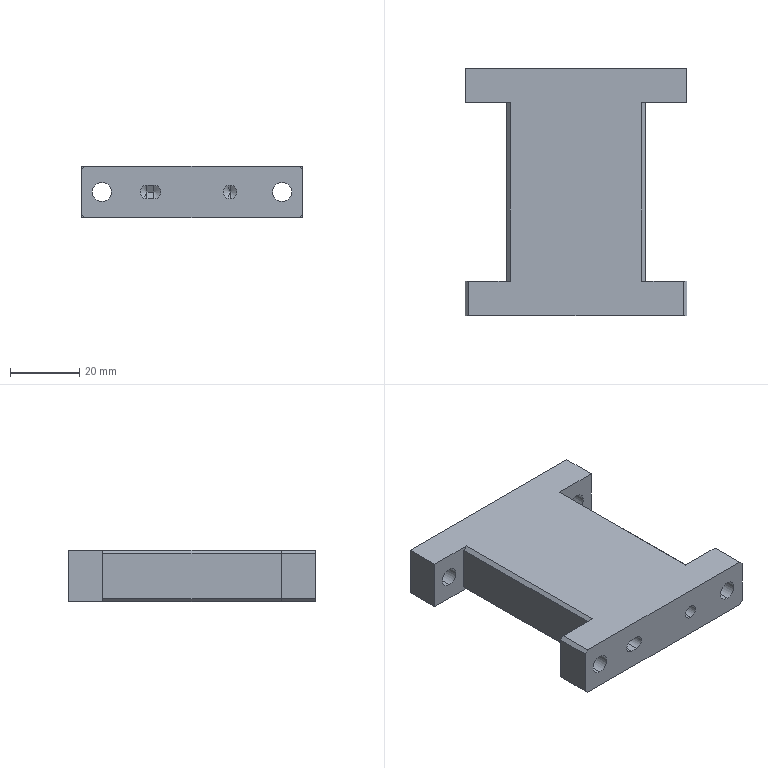Part | STEP file | 11-FG-GD00111 | 1 solid | 42 faces | box 64 x 71.5 x 15 mm | volume 48677 mm3 | plane 26 | cylinder 12 | cone 4 | commonest cylinder face diameters 5.5 x8 4 x4
STEP:
#1=CARTESIAN_POINT('',(26.,35.75,10.25));
#2=VERTEX_POINT('',#1);
#3=CARTESIAN_POINT('',(26.,35.75,4.75));
#4=VERTEX_POINT('',#3);
#5=CARTESIAN_POINT('',(26.,35.75,7.5));
#6=DIRECTION('',(0.,-1.,0.));
#7=DIRECTION('',(0.,0.,-1.));
#8=AXIS2_PLACEMENT_3D('',#5,#6,#7);
#9=CIRCLE('',#8,2.75);
#10=EDGE_CURVE('',#2,#4,#9,.T.);
#11=ORIENTED_EDGE('',*,*,#10,.F.);
#12=CARTESIAN_POINT('',(26.,25.75,10.25));
#13=VERTEX_POINT('',#12);
#14=CARTESIAN_POINT('',(26.,35.75,10.25));
#15=DIRECTION('',(0.,-1.,0.));
#16=VECTOR('',#15,1000.);
#17=LINE('',#14,#16);
#18=EDGE_CURVE('',#2,#13,#17,.T.);
#19=ORIENTED_EDGE('',*,*,#18,.T.);
#20=CARTESIAN_POINT('',(26.,25.75,4.75));
#21=VERTEX_POINT('',#20);
#22=CARTESIAN_POINT('',(26.,25.75,7.5));
#23=DIRECTION('',(0.,-1.,0.));
#24=DIRECTION('',(0.,0.,-1.));
#25=AXIS2_PLACEMENT_3D('',#22,#23,#24);
#26=CIRCLE('',#25,2.75);
#27=EDGE_CURVE('',#13,#21,#26,.T.);
#28=ORIENTED_EDGE('',*,*,#27,.T.);
#29=CARTESIAN_POINT('',(26.,35.75,4.75));
#30=DIRECTION('',(0.,-1.,0.));
#31=VECTOR('',#30,1000.);
#32=LINE('',#29,#31);
#33=EDGE_CURVE('',#4,#21,#32,.T.);
#34=ORIENTED_EDGE('',*,*,#33,.F.);
#35=EDGE_LOOP('',(#11,#19,#28,#34));
#36=FACE_OUTER_BOUND('',#35,.T.);
#37=CARTESIAN_POINT('',(26.,35.75,7.5));
#38=DIRECTION('',(0.,-1.,0.));
#39=DIRECTION('',(0.,0.,-1.));
#40=AXIS2_PLACEMENT_3D('',#37,#38,#39);
#41=CYLINDRICAL_SURFACE('',#40,2.75);
#42=ADVANCED_FACE('',(#36),#41,.F.);
#43=CARTESIAN_POINT('',(-26.,35.75,10.25));
#44=VERTEX_POINT('',#43);
#45=CARTESIAN_POINT('',(-26.,35.75,4.75));
#46=VERTEX_POINT('',#45);
#47=CARTESIAN_POINT('',(-26.,35.75,7.5));
#48=DIRECTION('',(0.,-1.,0.));
#49=DIRECTION('',(0.,0.,-1.));
#50=AXIS2_PLACEMENT_3D('',#47,#48,#49);
#51=CIRCLE('',#50,2.75);
#52=EDGE_CURVE('',#44,#46,#51,.T.);
#53=ORIENTED_EDGE('',*,*,#52,.F.);
#54=CARTESIAN_POINT('',(-26.,25.75,10.25));
#55=VERTEX_POINT('',#54);
#56=CARTESIAN_POINT('',(-26.,35.75,10.25));
#57=DIRECTION('',(0.,-1.,0.));
#58=VECTOR('',#57,1000.);
#59=LINE('',#56,#58);
#60=EDGE_CURVE('',#44,#55,#59,.T.);
#61=ORIENTED_EDGE('',*,*,#60,.T.);
#62=CARTESIAN_POINT('',(-26.,25.75,4.75));
#63=VERTEX_POINT('',#62);
#64=CARTESIAN_POINT('',(-26.,25.75,7.5));
#65=DIRECTION('',(0.,-1.,0.));
#66=DIRECTION('',(0.,0.,-1.));
#67=AXIS2_PLACEMENT_3D('',#64,#65,#66);
#68=CIRCLE('',#67,2.75);
#69=EDGE_CURVE('',#55,#63,#68,.T.);
#70=ORIENTED_EDGE('',*,*,#69,.T.);
#71=CARTESIAN_POINT('',(-26.,35.75,4.75));
#72=DIRECTION('',(0.,-1.,0.));
#73=VECTOR('',#72,1000.);
#74=LINE('',#71,#73);
#75=EDGE_CURVE('',#46,#63,#74,.T.);
#76=ORIENTED_EDGE('',*,*,#75,.F.);
#77=EDGE_LOOP('',(#53,#61,#70,#76));
#78=FACE_OUTER_BOUND('',#77,.T.);
#79=CARTESIAN_POINT('',(-26.,35.75,7.5));
#80=DIRECTION('',(0.,-1.,0.));
#81=DIRECTION('',(0.,0.,-1.));
#82=AXIS2_PLACEMENT_3D('',#79,#80,#81);
#83=CYLINDRICAL_SURFACE('',#82,2.75);
#84=ADVANCED_FACE('',(#78),#83,.F.);
#85=CARTESIAN_POINT('',(11.,-25.65,9.5));
#86=VERTEX_POINT('',#85);
#87=CARTESIAN_POINT('',(11.,-25.65,5.5));
#88=VERTEX_POINT('',#87);
#89=CARTESIAN_POINT('',(11.,-25.65,7.5));
#90=DIRECTION('',(0.,-1.,0.));
#91=DIRECTION('',(0.,0.,-1.));
#92=AXIS2_PLACEMENT_3D('',#89,#90,#91);
#93=CIRCLE('',#92,2.);
#94=EDGE_CURVE('',#86,#88,#93,.T.);
#95=ORIENTED_EDGE('',*,*,#94,.F.);
#96=CARTESIAN_POINT('',(11.,-35.75,9.5));
#97=VERTEX_POINT('',#96);
#98=CARTESIAN_POINT('',(11.,-35.75,9.5));
#99=DIRECTION('',(0.,-1.,0.));
#100=VECTOR('',#99,1000.);
#101=LINE('',#98,#100);
#102=EDGE_CURVE('',#86,#97,#101,.T.);
#103=ORIENTED_EDGE('',*,*,#102,.T.);
#104=CARTESIAN_POINT('',(11.,-35.75,5.5));
#105=VERTEX_POINT('',#104);
#106=CARTESIAN_POINT('',(11.,-35.75,7.5));
#107=DIRECTION('',(0.,-1.,0.));
#108=DIRECTION('',(0.,0.,-1.));
#109=AXIS2_PLACEMENT_3D('',#106,#107,#108);
#110=CIRCLE('',#109,2.);
#111=EDGE_CURVE('',#97,#105,#110,.T.);
#112=ORIENTED_EDGE('',*,*,#111,.T.);
#113=CARTESIAN_POINT('',(11.,-35.75,5.5));
#114=DIRECTION('',(0.,-1.,0.));
#115=VECTOR('',#114,1000.);
#116=LINE('',#113,#115);
#117=EDGE_CURVE('',#88,#105,#116,.T.);
#118=ORIENTED_EDGE('',*,*,#117,.F.);
#119=EDGE_LOOP('',(#95,#103,#112,#118));
#120=FACE_OUTER_BOUND('',#119,.T.);
#121=CARTESIAN_POINT('',(11.,-35.75,7.5));
#122=DIRECTION('',(0.,-1.,0.));
#123=DIRECTION('',(0.,0.,-1.));
#124=AXIS2_PLACEMENT_3D('',#121,#122,#123);
#125=CYLINDRICAL_SURFACE('',#124,2.);
#126=ADVANCED_FACE('',(#120),#125,.F.);
#127=CARTESIAN_POINT('',(11.,-24.448,7.5));
#128=VERTEX_POINT('',#127);
#129=CARTESIAN_POINT('',(11.,-25.65,5.5));
#130=DIRECTION('',(0.,-0.515,-0.8572));
#131=VECTOR('',#130,1000.);
#132=LINE('',#129,#131);
#133=EDGE_CURVE('',#128,#88,#132,.T.);
#134=ORIENTED_EDGE('',*,*,#133,.F.);
#135=CARTESIAN_POINT('',(11.,-25.65,9.5));
#136=DIRECTION('',(0.,-0.515,0.8572));
#137=VECTOR('',#136,1000.);
#138=LINE('',#135,#137);
#139=EDGE_CURVE('',#128,#86,#138,.T.);
#140=ORIENTED_EDGE('',*,*,#139,.T.);
#141=ORIENTED_EDGE('',*,*,#94,.T.);
#142=EDGE_LOOP('',(#134,#140,#141));
#143=FACE_OUTER_BOUND('',#142,.T.);
#144=CARTESIAN_POINT('',(11.,-25.65,7.5));
#145=DIRECTION('',(0.,-1.,0.));
#146=DIRECTION('',(0.,0.,-1.));
#147=AXIS2_PLACEMENT_3D('',#144,#145,#146);
#148=CONICAL_SURFACE('',#147,2.,1.03);
#149=ADVANCED_FACE('',(#143),#148,.F.);
#150=CARTESIAN_POINT('',(26.,-35.75,4.75));
#151=VERTEX_POINT('',#150);
#152=CARTESIAN_POINT('',(26.,-35.75,10.25));
#153=VERTEX_POINT('',#152);
#154=CARTESIAN_POINT('',(26.,-35.75,7.5));
#155=DIRECTION('',(0.,1.,0.));
#156=DIRECTION('',(0.,0.,-1.));
#157=AXIS2_PLACEMENT_3D('',#154,#155,#156);
#158=CIRCLE('',#157,2.75);
#159=EDGE_CURVE('',#151,#153,#158,.T.);
#160=ORIENTED_EDGE('',*,*,#159,.F.);
#161=CARTESIAN_POINT('',(26.,-25.75,4.75));
#162=VERTEX_POINT('',#161);
#163=CARTESIAN_POINT('',(26.,-35.75,4.75));
#164=DIRECTION('',(0.,1.,0.));
#165=VECTOR('',#164,1000.);
#166=LINE('',#163,#165);
#167=EDGE_CURVE('',#151,#162,#166,.T.);
#168=ORIENTED_EDGE('',*,*,#167,.T.);
#169=CARTESIAN_POINT('',(26.,-25.75,10.25));
#170=VERTEX_POINT('',#169);
#171=CARTESIAN_POINT('',(26.,-25.75,7.5));
#172=DIRECTION('',(0.,1.,0.));
#173=DIRECTION('',(0.,0.,-1.));
#174=AXIS2_PLACEMENT_3D('',#171,#172,#173);
#175=CIRCLE('',#174,2.75);
#176=EDGE_CURVE('',#162,#170,#175,.T.);
#177=ORIENTED_EDGE('',*,*,#176,.T.);
#178=CARTESIAN_POINT('',(26.,-35.75,10.25));
#179=DIRECTION('',(0.,1.,0.));
#180=VECTOR('',#179,1000.);
#181=LINE('',#178,#180);
#182=EDGE_CURVE('',#153,#170,#181,.T.);
#183=ORIENTED_EDGE('',*,*,#182,.F.);
#184=EDGE_LOOP('',(#160,#168,#177,#183));
#185=FACE_OUTER_BOUND('',#184,.T.);
#186=CARTESIAN_POINT('',(26.,-35.75,7.5));
#187=DIRECTION('',(0.,1.,0.));
#188=DIRECTION('',(0.,0.,1.));
#189=AXIS2_PLACEMENT_3D('',#186,#187,#188);
#190=CYLINDRICAL_SURFACE('',#189,2.75);
#191=ADVANCED_FACE('',(#185),#190,.F.);
#192=CARTESIAN_POINT('',(-26.,-35.75,4.75));
#193=VERTEX_POINT('',#192);
#194=CARTESIAN_POINT('',(-26.,-35.75,10.25));
#195=VERTEX_POINT('',#194);
#196=CARTESIAN_POINT('',(-26.,-35.75,7.5));
#197=DIRECTION('',(0.,1.,0.));
#198=DIRECTION('',(0.,0.,1.));
#199=AXIS2_PLACEMENT_3D('',#196,#197,#198);
#200=CIRCLE('',#199,2.75);
#201=EDGE_CURVE('',#193,#195,#200,.T.);
#202=ORIENTED_EDGE('',*,*,#201,.F.);
#203=CARTESIAN_POINT('',(-26.,-25.75,4.75));
#204=VERTEX_POINT('',#203);
#205=CARTESIAN_POINT('',(-26.,-35.75,4.75));
#206=DIRECTION('',(0.,1.,0.));
#207=VECTOR('',#206,1000.);
#208=LINE('',#205,#207);
#209=EDGE_CURVE('',#193,#204,#208,.T.);
#210=ORIENTED_EDGE('',*,*,#209,.T.);
#211=CARTESIAN_POINT('',(-26.,-25.75,10.25));
#212=VERTEX_POINT('',#211);
#213=CARTESIAN_POINT('',(-26.,-25.75,7.5));
#214=DIRECTION('',(0.,1.,0.));
#215=DIRECTION('',(0.,0.,1.));
#216=AXIS2_PLACEMENT_3D('',#213,#214,#215);
#217=CIRCLE('',#216,2.75);
#218=EDGE_CURVE('',#204,#212,#217,.T.);
#219=ORIENTED_EDGE('',*,*,#218,.T.);
#220=CARTESIAN_POINT('',(-26.,-35.75,10.25));
#221=DIRECTION('',(0.,1.,0.));
#222=VECTOR('',#221,1000.);
#223=LINE('',#220,#222);
#224=EDGE_CURVE('',#195,#212,#223,.T.);
#225=ORIENTED_EDGE('',*,*,#224,.F.);
#226=EDGE_LOOP('',(#202,#210,#219,#225));
#227=FACE_OUTER_BOUND('',#226,.T.);
#228=CARTESIAN_POINT('',(-26.,-35.75,7.5));
#229=DIRECTION('',(0.,1.,0.));
#230=DIRECTION('',(0.,0.,1.));
#231=AXIS2_PLACEMENT_3D('',#228,#229,#230);
#232=CYLINDRICAL_SURFACE('',#231,2.75);
#233=ADVANCED_FACE('',(#227),#232,.F.);
#234=CARTESIAN_POINT('',(20.,25.75,1.));
#235=VERTEX_POINT('',#234);
#236=CARTESIAN_POINT('',(20.,25.75,14.));
#237=VERTEX_POINT('',#236);
#238=CARTESIAN_POINT('',(20.,25.75,0.));
#239=DIRECTION('',(0.,0.,1.));
#240=VECTOR('',#239,1000.);
#241=LINE('',#238,#240);
#242=EDGE_CURVE('',#235,#237,#241,.T.);
#243=ORIENTED_EDGE('',*,*,#242,.T.);
#244=CARTESIAN_POINT('',(20.,-25.75,14.));
#245=VERTEX_POINT('',#244);
#246=CARTESIAN_POINT('',(20.,-25.75,14.));
#247=DIRECTION('',(0.,-1.,0.));
#248=VECTOR('',#247,1000.);
#249=LINE('',#246,#248);
#250=EDGE_CURVE('',#237,#245,#249,.T.);
#251=ORIENTED_EDGE('',*,*,#250,.T.);
#252=CARTESIAN_POINT('',(20.,-25.75,1.));
#253=VERTEX_POINT('',#252);
#254=CARTESIAN_POINT('',(20.,-25.75,0.));
#255=DIRECTION('',(0.,0.,1.));
#256=VECTOR('',#255,1000.);
#257=LINE('',#254,#256);
#258=EDGE_CURVE('',#253,#245,#257,.T.);
#259=ORIENTED_EDGE('',*,*,#258,.F.);
#260=CARTESIAN_POINT('',(20.,35.75,1.));
#261=DIRECTION('',(0.,1.,0.));
#262=VECTOR('',#261,1000.);
#263=LINE('',#260,#262);
#264=EDGE_CURVE('',#253,#235,#263,.T.);
#265=ORIENTED_EDGE('',*,*,#264,.T.);
#266=EDGE_LOOP('',(#243,#251,#259,#265));
#267=FACE_OUTER_BOUND('',#266,.T.);
#268=CARTESIAN_POINT('',(20.,35.75,15.));
#269=DIRECTION('',(-1.,0.,0.));
#270=DIRECTION('',(0.,-1.,0.));
#271=AXIS2_PLACEMENT_3D('',#268,#269,#270);
#272=PLANE('',#271);
#273=ADVANCED_FACE('',(#267),#272,.F.);
#274=CARTESIAN_POINT('',(26.,35.75,7.5));
#275=DIRECTION('',(0.,-1.,0.));
#276=DIRECTION('',(0.,0.,-1.));
#277=AXIS2_PLACEMENT_3D('',#274,#275,#276);
#278=CIRCLE('',#277,2.75);
#279=EDGE_CURVE('',#4,#2,#278,.T.);
#280=ORIENTED_EDGE('',*,*,#279,.T.);
#281=ORIENTED_EDGE('',*,*,#10,.T.);
#282=EDGE_LOOP('',(#280,#281));
#283=FACE_BOUND('',#282,.T.);
#284=CARTESIAN_POINT('',(-26.,35.75,7.5));
#285=DIRECTION('',(0.,-1.,0.));
#286=DIRECTION('',(0.,0.,-1.));
#287=AXIS2_PLACEMENT_3D('',#284,#285,#286);
#288=CIRCLE('',#287,2.75);
#289=EDGE_CURVE('',#46,#44,#288,.T.);
#290=ORIENTED_EDGE('',*,*,#289,.T.);
#291=ORIENTED_EDGE('',*,*,#52,.T.);
#292=EDGE_LOOP('',(#290,#291));
#293=FACE_BOUND('',#292,.T.);
#294=CARTESIAN_POINT('',(32.,35.75,0.));
#295=VERTEX_POINT('',#294);
#296=CARTESIAN_POINT('',(-32.,35.75,0.));
#297=VERTEX_POINT('',#296);
#298=CARTESIAN_POINT('',(-20.,35.75,0.));
#299=DIRECTION('',(-1.,0.,0.));
#300=VECTOR('',#299,1000.);
#301=LINE('',#298,#300);
#302=EDGE_CURVE('',#295,#297,#301,.T.);
#303=ORIENTED_EDGE('',*,*,#302,.T.);
#304=CARTESIAN_POINT('',(-32.,35.75,15.));
#305=VERTEX_POINT('',#304);
#306=CARTESIAN_POINT('',(-32.,35.75,0.));
#307=DIRECTION('',(0.,0.,1.));
#308=VECTOR('',#307,1000.);
#309=LINE('',#306,#308);
#310=EDGE_CURVE('',#297,#305,#309,.T.);
#311=ORIENTED_EDGE('',*,*,#310,.T.);
#312=CARTESIAN_POINT('',(32.,35.75,15.));
#313=VERTEX_POINT('',#312);
#314=CARTESIAN_POINT('',(-20.,35.75,15.));
#315=DIRECTION('',(-1.,0.,0.));
#316=VECTOR('',#315,1000.);
#317=LINE('',#314,#316);
#318=EDGE_CURVE('',#313,#305,#317,.T.);
#319=ORIENTED_EDGE('',*,*,#318,.F.);
#320=CARTESIAN_POINT('',(32.,35.75,0.));
#321=DIRECTION('',(0.,0.,1.));
#322=VECTOR('',#321,1000.);
#323=LINE('',#320,#322);
#324=EDGE_CURVE('',#295,#313,#323,.T.);
#325=ORIENTED_EDGE('',*,*,#324,.F.);
#326=EDGE_LOOP('',(#303,#311,#319,#325));
#327=FACE_OUTER_BOUND('',#326,.T.);
#328=CARTESIAN_POINT('',(-20.,35.75,15.));
#329=DIRECTION('',(0.,-1.,0.));
#330=DIRECTION('',(0.,0.,-1.));
#331=AXIS2_PLACEMENT_3D('',#328,#329,#330);
#332=PLANE('',#331);
#333=ADVANCED_FACE('',(#283,#293,#327),#332,.F.);
#334=CARTESIAN_POINT('',(-20.,-25.75,1.));
#335=VERTEX_POINT('',#334);
#336=CARTESIAN_POINT('',(-20.,-25.75,14.));
#337=VERTEX_POINT('',#336);
#338=CARTESIAN_POINT('',(-20.,-25.75,0.));
#339=DIRECTION('',(0.,0.,1.));
#340=VECTOR('',#339,1000.);
#341=LINE('',#338,#340);
#342=EDGE_CURVE('',#335,#337,#341,.T.);
#343=ORIENTED_EDGE('',*,*,#342,.T.);
#344=CARTESIAN_POINT('',(-20.,25.75,14.));
#345=VERTEX_POINT('',#344);
#346=CARTESIAN_POINT('',(-20.,25.75,14.));
#347=DIRECTION('',(0.,1.,0.));
#348=VECTOR('',#347,1000.);
#349=LINE('',#346,#348);
#350=EDGE_CURVE('',#337,#345,#349,.T.);
#351=ORIENTED_EDGE('',*,*,#350,.T.);
#352=CARTESIAN_POINT('',(-20.,25.75,1.));
#353=VERTEX_POINT('',#352);
#354=CARTESIAN_POINT('',(-20.,25.75,0.));
#355=DIRECTION('',(0.,0.,1.));
#356=VECTOR('',#355,1000.);
#357=LINE('',#354,#356);
#358=EDGE_CURVE('',#353,#345,#357,.T.);
#359=ORIENTED_EDGE('',*,*,#358,.F.);
#360=CARTESIAN_POINT('',(-20.,35.75,1.));
#361=DIRECTION('',(0.,-1.,0.));
#362=VECTOR('',#361,1000.);
#363=LINE('',#360,#362);
#364=EDGE_CURVE('',#353,#335,#363,.T.);
#365=ORIENTED_EDGE('',*,*,#364,.T.);
#366=EDGE_LOOP('',(#343,#351,#359,#365));
#367=FACE_OUTER_BOUND('',#366,.T.);
#368=CARTESIAN_POINT('',(-20.,35.75,15.));
#369=DIRECTION('',(1.,0.,0.));
#370=DIRECTION('',(0.,1.,0.));
#371=AXIS2_PLACEMENT_3D('',#368,#369,#370);
#372=PLANE('',#371);
#373=ADVANCED_FACE('',(#367),#372,.F.);
#374=CARTESIAN_POINT('',(-13.,-35.75,9.5));
#375=VERTEX_POINT('',#374);
#376=CARTESIAN_POINT('',(-13.,-35.75,5.5));
#377=VERTEX_POINT('',#376);
#378=CARTESIAN_POINT('',(-13.,-35.75,7.5));
#379=DIRECTION('',(0.,-1.,0.));
#380=DIRECTION('',(0.,0.,-1.));
#381=AXIS2_PLACEMENT_3D('',#378,#379,#380);
#382=CIRCLE('',#381,2.);
#383=EDGE_CURVE('',#375,#377,#382,.T.);
#384=ORIENTED_EDGE('',*,*,#383,.F.);
#385=CARTESIAN_POINT('',(-11.,-35.75,9.5));
#386=VERTEX_POINT('',#385);
#387=CARTESIAN_POINT('',(-13.,-35.75,9.5));
#388=DIRECTION('',(1.,0.,0.));
#389=VECTOR('',#388,1000.);
#390=LINE('',#387,#389);
#391=EDGE_CURVE('',#375,#386,#390,.T.);
#392=ORIENTED_EDGE('',*,*,#391,.T.);
#393=CARTESIAN_POINT('',(-11.,-35.75,5.5));
#394=VERTEX_POINT('',#393);
#395=CARTESIAN_POINT('',(-11.,-35.75,7.5));
#396=DIRECTION('',(0.,-1.,0.));
#397=DIRECTION('',(0.,0.,-1.));
#398=AXIS2_PLACEMENT_3D('',#395,#396,#397);
#399=CIRCLE('',#398,2.);
#400=EDGE_CURVE('',#394,#386,#399,.T.);
#401=ORIENTED_EDGE('',*,*,#400,.F.);
#402=CARTESIAN_POINT('',(-13.,-35.75,5.5));
#403=DIRECTION('',(1.,0.,0.));
#404=VECTOR('',#403,1000.);
#405=LINE('',#402,#404);
#406=EDGE_CURVE('',#377,#394,#405,.T.);
#407=ORIENTED_EDGE('',*,*,#406,.F.);
#408=EDGE_LOOP('',(#384,#392,#401,#407));
#409=FACE_BOUND('',#408,.T.);
#410=CARTESIAN_POINT('',(11.,-35.75,7.5));
#411=DIRECTION('',(0.,-1.,0.));
#412=DIRECTION('',(0.,0.,-1.));
#413=AXIS2_PLACEMENT_3D('',#410,#411,#412);
#414=CIRCLE('',#413,2.);
#415=EDGE_CURVE('',#105,#97,#414,.T.);
#416=ORIENTED_EDGE('',*,*,#415,.F.);
#417=ORIENTED_EDGE('',*,*,#111,.F.);
#418=EDGE_LOOP('',(#416,#417));
#419=FACE_BOUND('',#418,.T.);
#420=CARTESIAN_POINT('',(26.,-35.75,7.5));
#421=DIRECTION('',(0.,1.,0.));
#422=DIRECTION('',(0.,0.,-1.));
#423=AXIS2_PLACEMENT_3D('',#420,#421,#422);
#424=CIRCLE('',#423,2.75);
#425=EDGE_CURVE('',#153,#151,#424,.T.);
#426=ORIENTED_EDGE('',*,*,#425,.T.);
#427=ORIENTED_EDGE('',*,*,#159,.T.);
#428=EDGE_LOOP('',(#426,#427));
#429=FACE_BOUND('',#428,.T.);
#430=CARTESIAN_POINT('',(-26.,-35.75,7.5));
#431=DIRECTION('',(0.,1.,0.));
#432=DIRECTION('',(0.,0.,1.));
#433=AXIS2_PLACEMENT_3D('',#430,#431,#432);
#434=CIRCLE('',#433,2.75);
#435=EDGE_CURVE('',#195,#193,#434,.T.);
#436=ORIENTED_EDGE('',*,*,#435,.T.);
#437=ORIENTED_EDGE('',*,*,#201,.T.);
#438=EDGE_LOOP('',(#436,#437));
#439=FACE_BOUND('',#438,.T.);
#440=CARTESIAN_POINT('',(-32.,-35.75,1.));
#441=VERTEX_POINT('',#440);
#442=CARTESIAN_POINT('',(-32.,-35.75,14.));
#443=VERTEX_POINT('',#442);
#444=CARTESIAN_POINT('',(-32.,-35.75,0.));
#445=DIRECTION('',(0.,0.,1.));
#446=VECTOR('',#445,1000.);
#447=LINE('',#444,#446);
#448=EDGE_CURVE('',#441,#443,#447,.T.);
#449=ORIENTED_EDGE('',*,*,#448,.F.);
#450=CARTESIAN_POINT('',(-31.,-35.75,0.));
#451=VERTEX_POINT('',#450);
#452=CARTESIAN_POINT('',(-32.,-35.75,1.));
#453=DIRECTION('',(0.7071,0.,-0.7071));
#454=VECTOR('',#453,1000.);
#455=LINE('',#452,#454);
#456=EDGE_CURVE('',#441,#451,#455,.T.);
#457=ORIENTED_EDGE('',*,*,#456,.T.);
#458=CARTESIAN_POINT('',(31.,-35.75,0.));
#459=VERTEX_POINT('',#458);
#460=CARTESIAN_POINT('',(-20.,-35.75,0.));
#461=DIRECTION('',(1.,0.,0.));
#462=VECTOR('',#461,1000.);
#463=LINE('',#460,#462);
#464=EDGE_CURVE('',#451,#459,#463,.T.);
#465=ORIENTED_EDGE('',*,*,#464,.T.);
#466=CARTESIAN_POINT('',(32.,-35.75,1.));
#467=VERTEX_POINT('',#466);
#468=CARTESIAN_POINT('',(32.,-35.75,1.));
#469=DIRECTION('',(0.7071,0.,0.7071));
#470=VECTOR('',#469,1000.);
#471=LINE('',#468,#470);
#472=EDGE_CURVE('',#459,#467,#471,.T.);
#473=ORIENTED_EDGE('',*,*,#472,.T.);
#474=CARTESIAN_POINT('',(32.,-35.75,14.));
#475=VERTEX_POINT('',#474);
#476=CARTESIAN_POINT('',(32.,-35.75,0.));
#477=DIRECTION('',(0.,0.,1.));
#478=VECTOR('',#477,1000.);
#479=LINE('',#476,#478);
#480=EDGE_CURVE('',#467,#475,#479,.T.);
#481=ORIENTED_EDGE('',*,*,#480,.T.);
#482=CARTESIAN_POINT('',(31.,-35.75,15.));
#483=VERTEX_POINT('',#482);
#484=CARTESIAN_POINT('',(31.,-35.75,15.));
#485=DIRECTION('',(-0.7071,0.,0.7071));
#486=VECTOR('',#485,1000.);
#487=LINE('',#484,#486);
#488=EDGE_CURVE('',#475,#483,#487,.T.);
#489=ORIENTED_EDGE('',*,*,#488,.T.);
#490=CARTESIAN_POINT('',(-31.,-35.75,15.));
#491=VERTEX_POINT('',#490);
#492=CARTESIAN_POINT('',(-20.,-35.75,15.));
#493=DIRECTION('',(1.,0.,0.));
#494=VECTOR('',#493,1000.);
#495=LINE('',#492,#494);
#496=EDGE_CURVE('',#491,#483,#495,.T.);
#497=ORIENTED_EDGE('',*,*,#496,.F.);
#498=CARTESIAN_POINT('',(-31.,-35.75,15.));
#499=DIRECTION('',(-0.7071,0.,-0.7071));
#500=VECTOR('',#499,1000.);
#501=LINE('',#498,#500);
#502=EDGE_CURVE('',#491,#443,#501,.T.);
#503=ORIENTED_EDGE('',*,*,#502,.T.);
#504=EDGE_LOOP('',(#449,#457,#465,#473,#481,#489,#497,#503));
#505=FACE_OUTER_BOUND('',#504,.T.);
#506=CARTESIAN_POINT('',(-20.,-35.75,15.));
#507=DIRECTION('',(0.,1.,0.));
#508=DIRECTION('',(0.,0.,1.));
#509=AXIS2_PLACEMENT_3D('',#506,#507,#508);
#510=PLANE('',#509);
#511=ADVANCED_FACE('',(#409,#419,#429,#439,#505),#510,.F.);
#512=CARTESIAN_POINT('',(-19.,-25.75,15.));
#513=VERTEX_POINT('',#512);
#514=CARTESIAN_POINT('',(-31.,-25.75,15.));
#515=VERTEX_POINT('',#514);
#516=CARTESIAN_POINT('',(-20.,-25.75,15.));
#517=DIRECTION('',(-1.,0.,0.));
#518=VECTOR('',#517,1000.);
#519=LINE('',#516,#518);
#520=EDGE_CURVE('',#513,#515,#519,.T.);
#521=ORIENTED_EDGE('',*,*,#520,.T.);
#522=CARTESIAN_POINT('',(-31.,0.,15.));
#523=DIRECTION('',(0.,-1.,0.));
#524=VECTOR('',#523,1000.);
#525=LINE('',#522,#524);
#526=EDGE_CURVE('',#515,#491,#525,.T.);
#527=ORIENTED_EDGE('',*,*,#526,.T.);
#528=ORIENTED_EDGE('',*,*,#496,.T.);
#529=CARTESIAN_POINT('',(31.,-25.75,15.));
#530=VERTEX_POINT('',#529);
#531=CARTESIAN_POINT('',(31.,0.,15.));
#532=DIRECTION('',(0.,1.,0.));
#533=VECTOR('',#532,1000.);
#534=LINE('',#531,#533);
#535=EDGE_CURVE('',#483,#530,#534,.T.);
#536=ORIENTED_EDGE('',*,*,#535,.T.);
#537=CARTESIAN_POINT('',(19.,-25.75,15.));
#538=VERTEX_POINT('',#537);
#539=CARTESIAN_POINT('',(20.,-25.75,15.));
#540=DIRECTION('',(-1.,0.,0.));
#541=VECTOR('',#540,1000.);
#542=LINE('',#539,#541);
#543=EDGE_CURVE('',#530,#538,#542,.T.);
#544=ORIENTED_EDGE('',*,*,#543,.T.);
#545=CARTESIAN_POINT('',(19.,25.75,15.));
#546=VERTEX_POINT('',#545);
#547=CARTESIAN_POINT('',(19.,25.75,15.));
#548=DIRECTION('',(0.,1.,0.));
#549=VECTOR('',#548,1000.);
#550=LINE('',#547,#549);
#551=EDGE_CURVE('',#538,#546,#550,.T.);
#552=ORIENTED_EDGE('',*,*,#551,.T.);
#553=CARTESIAN_POINT('',(32.,25.75,15.));
#554=VERTEX_POINT('',#553);
#555=CARTESIAN_POINT('',(20.,25.75,15.));
#556=DIRECTION('',(1.,0.,0.));
#557=VECTOR('',#556,1000.);
#558=LINE('',#555,#557);
#559=EDGE_CURVE('',#546,#554,#558,.T.);
#560=ORIENTED_EDGE('',*,*,#559,.T.);
#561=CARTESIAN_POINT('',(32.,35.75,15.));
#562=DIRECTION('',(0.,1.,0.));
#563=VECTOR('',#562,1000.);
#564=LINE('',#561,#563);
#565=EDGE_CURVE('',#554,#313,#564,.T.);
#566=ORIENTED_EDGE('',*,*,#565,.T.);
#567=ORIENTED_EDGE('',*,*,#318,.T.);
#568=CARTESIAN_POINT('',(-32.,25.75,15.));
#569=VERTEX_POINT('',#568);
#570=CARTESIAN_POINT('',(-32.,35.75,15.));
#571=DIRECTION('',(0.,-1.,0.));
#572=VECTOR('',#571,1000.);
#573=LINE('',#570,#572);
#574=EDGE_CURVE('',#305,#569,#573,.T.);
#575=ORIENTED_EDGE('',*,*,#574,.T.);
#576=CARTESIAN_POINT('',(-19.,25.75,15.));
#577=VERTEX_POINT('',#576);
#578=CARTESIAN_POINT('',(-20.,25.75,15.));
#579=DIRECTION('',(1.,0.,0.));
#580=VECTOR('',#579,1000.);
#581=LINE('',#578,#580);
#582=EDGE_CURVE('',#569,#577,#581,.T.);
#583=ORIENTED_EDGE('',*,*,#582,.T.);
#584=CARTESIAN_POINT('',(-19.,-25.75,15.));
#585=DIRECTION('',(0.,-1.,0.));
#586=VECTOR('',#585,1000.);
#587=LINE('',#584,#586);
#588=EDGE_CURVE('',#577,#513,#587,.T.);
#589=ORIENTED_EDGE('',*,*,#588,.T.);
#590=EDGE_LOOP('',(#521,#527,#528,#536,#544,#552,#560,#566,#567,#575,#583,#589));
#591=FACE_OUTER_BOUND('',#590,.T.);
#592=CARTESIAN_POINT('',(0.,0.,15.));
#593=DIRECTION('',(0.,0.,1.));
#594=DIRECTION('',(1.,0.,0.));
#595=AXIS2_PLACEMENT_3D('',#592,#593,#594);
#596=PLANE('',#595);
#597=ADVANCED_FACE('',(#591),#596,.T.);
#598=ORIENTED_EDGE('',*,*,#464,.F.);
#599=CARTESIAN_POINT('',(-31.,-25.75,0.));
#600=VERTEX_POINT('',#599);
#601=CARTESIAN_POINT('',(-31.,-25.75,0.));
#602=DIRECTION('',(0.,1.,0.));
#603=VECTOR('',#602,1000.);
#604=LINE('',#601,#603);
#605=EDGE_CURVE('',#451,#600,#604,.T.);
#606=ORIENTED_EDGE('',*,*,#605,.T.);
#607=CARTESIAN_POINT('',(-19.,-25.75,0.));
#608=VERTEX_POINT('',#607);
#609=CARTESIAN_POINT('',(-20.,-25.75,0.));
#610=DIRECTION('',(-1.,0.,0.));
#611=VECTOR('',#610,1000.);
#612=LINE('',#609,#611);
#613=EDGE_CURVE('',#608,#600,#612,.T.);
#614=ORIENTED_EDGE('',*,*,#613,.F.);
#615=CARTESIAN_POINT('',(-19.,25.75,0.));
#616=VERTEX_POINT('',#615);
#617=CARTESIAN_POINT('',(-19.,0.,0.));
#618=DIRECTION('',(0.,1.,0.));
#619=VECTOR('',#618,1000.);
#620=LINE('',#617,#619);
#621=EDGE_CURVE('',#608,#616,#620,.T.);
#622=ORIENTED_EDGE('',*,*,#621,.T.);
#623=CARTESIAN_POINT('',(-32.,25.75,0.));
#624=VERTEX_POINT('',#623);
#625=CARTESIAN_POINT('',(-20.,25.75,0.));
#626=DIRECTION('',(1.,0.,0.));
#627=VECTOR('',#626,1000.);
#628=LINE('',#625,#627);
#629=EDGE_CURVE('',#624,#616,#628,.T.);
#630=ORIENTED_EDGE('',*,*,#629,.F.);
#631=CARTESIAN_POINT('',(-32.,35.75,0.));
#632=DIRECTION('',(0.,-1.,0.));
#633=VECTOR('',#632,1000.);
#634=LINE('',#631,#633);
#635=EDGE_CURVE('',#297,#624,#634,.T.);
#636=ORIENTED_EDGE('',*,*,#635,.F.);
#637=ORIENTED_EDGE('',*,*,#302,.F.);
#638=CARTESIAN_POINT('',(32.,25.75,0.));
#639=VERTEX_POINT('',#638);
#640=CARTESIAN_POINT('',(32.,35.75,0.));
#641=DIRECTION('',(0.,1.,0.));
#642=VECTOR('',#641,1000.);
#643=LINE('',#640,#642);
#644=EDGE_CURVE('',#639,#295,#643,.T.);
#645=ORIENTED_EDGE('',*,*,#644,.F.);
#646=CARTESIAN_POINT('',(19.,25.75,0.));
#647=VERTEX_POINT('',#646);
#648=CARTESIAN_POINT('',(20.,25.75,0.));
#649=DIRECTION('',(1.,0.,0.));
#650=VECTOR('',#649,1000.);
#651=LINE('',#648,#650);
#652=EDGE_CURVE('',#647,#639,#651,.T.);
#653=ORIENTED_EDGE('',*,*,#652,.F.);
#654=CARTESIAN_POINT('',(19.,-25.75,0.));
#655=VERTEX_POINT('',#654);
#656=CARTESIAN_POINT('',(19.,0.,0.));
#657=DIRECTION('',(0.,-1.,0.));
#658=VECTOR('',#657,1000.);
#659=LINE('',#656,#658);
#660=EDGE_CURVE('',#647,#655,#659,.T.);
#661=ORIENTED_EDGE('',*,*,#660,.T.);
#662=CARTESIAN_POINT('',(31.,-25.75,0.));
#663=VERTEX_POINT('',#662);
#664=CARTESIAN_POINT('',(20.,-25.75,0.));
#665=DIRECTION('',(-1.,0.,0.));
#666=VECTOR('',#665,1000.);
#667=LINE('',#664,#666);
#668=EDGE_CURVE('',#663,#655,#667,.T.);
#669=ORIENTED_EDGE('',*,*,#668,.F.);
#670=CARTESIAN_POINT('',(31.,-35.75,0.));
#671=DIRECTION('',(0.,-1.,0.));
#672=VECTOR('',#671,1000.);
#673=LINE('',#670,#672);
#674=EDGE_CURVE('',#663,#459,#673,.T.);
#675=ORIENTED_EDGE('',*,*,#674,.T.);
#676=EDGE_LOOP('',(#598,#606,#614,#622,#630,#636,#637,#645,#653,#661,#669,#675));
#677=FACE_OUTER_BOUND('',#676,.T.);
#678=CARTESIAN_POINT('',(0.,0.,0.));
#679=DIRECTION('',(0.,0.,1.));
#680=DIRECTION('',(1.,0.,0.));
#681=AXIS2_PLACEMENT_3D('',#678,#679,#680);
#682=PLANE('',#681);
#683=ADVANCED_FACE('',(#677),#682,.F.);
#684=CARTESIAN_POINT('',(-32.,-25.75,1.));
#685=VERTEX_POINT('',#684);
#686=CARTESIAN_POINT('',(-32.,-25.75,14.));
#687=VERTEX_POINT('',#686);
#688=CARTESIAN_POINT('',(-32.,-25.75,0.));
#689=DIRECTION('',(0.,0.,1.));
#690=VECTOR('',#689,1000.);
#691=LINE('',#688,#690);
#692=EDGE_CURVE('',#685,#687,#691,.T.);
#693=ORIENTED_EDGE('',*,*,#692,.F.);
#694=CARTESIAN_POINT('',(-32.,-35.75,1.));
#695=DIRECTION('',(0.,-1.,0.));
#696=VECTOR('',#695,1000.);
#697=LINE('',#694,#696);
#698=EDGE_CURVE('',#685,#441,#697,.T.);
#699=ORIENTED_EDGE('',*,*,#698,.T.);
#700=ORIENTED_EDGE('',*,*,#448,.T.);
#701=CARTESIAN_POINT('',(-32.,-35.75,14.));
#702=DIRECTION('',(0.,1.,0.));
#703=VECTOR('',#702,1000.);
#704=LINE('',#701,#703);
#705=EDGE_CURVE('',#443,#687,#704,.T.);
#706=ORIENTED_EDGE('',*,*,#705,.T.);
#707=EDGE_LOOP('',(#693,#699,#700,#706));
#708=FACE_OUTER_BOUND('',#707,.T.);
#709=CARTESIAN_POINT('',(-32.,-35.75,0.));
#710=DIRECTION('',(-1.,0.,0.));
#711=DIRECTION('',(0.,0.,1.));
#712=AXIS2_PLACEMENT_3D('',#709,#710,#711);
#713=PLANE('',#712);
#714=ADVANCED_FACE('',(#708),#713,.T.);
#715=CARTESIAN_POINT('',(-26.,-25.75,7.5));
#716=DIRECTION('',(0.,1.,0.));
#717=DIRECTION('',(0.,0.,1.));
#718=AXIS2_PLACEMENT_3D('',#715,#716,#717);
#719=CIRCLE('',#718,2.75);
#720=EDGE_CURVE('',#212,#204,#719,.T.);
#721=ORIENTED_EDGE('',*,*,#720,.F.);
#722=ORIENTED_EDGE('',*,*,#218,.F.);
#723=EDGE_LOOP('',(#721,#722));
#724=FACE_BOUND('',#723,.T.);
#725=ORIENTED_EDGE('',*,*,#613,.T.);
#726=CARTESIAN_POINT('',(-25.5,-25.75,-5.5));
#727=DIRECTION('',(-0.7071,0.,0.7071));
#728=VECTOR('',#727,1000.);
#729=LINE('',#726,#728);
#730=EDGE_CURVE('',#600,#685,#729,.T.);
#731=ORIENTED_EDGE('',*,*,#730,.T.);
#732=ORIENTED_EDGE('',*,*,#692,.T.);
#733=CARTESIAN_POINT('',(-33.,-25.75,13.));
#734=DIRECTION('',(0.7071,0.,0.7071));
#735=VECTOR('',#734,1000.);
#736=LINE('',#733,#735);
#737=EDGE_CURVE('',#687,#515,#736,.T.);
#738=ORIENTED_EDGE('',*,*,#737,.T.);
#739=ORIENTED_EDGE('',*,*,#520,.F.);
#740=CARTESIAN_POINT('',(-19.,-25.75,15.));
#741=DIRECTION('',(-0.7071,0.,-0.7071));
#742=VECTOR('',#741,1000.);
#743=LINE('',#740,#742);
#744=EDGE_CURVE('',#513,#337,#743,.T.);
#745=ORIENTED_EDGE('',*,*,#744,.T.);
#746=ORIENTED_EDGE('',*,*,#342,.F.);
#747=CARTESIAN_POINT('',(-20.,-25.75,1.));
#748=DIRECTION('',(0.7071,0.,-0.7071));
#749=VECTOR('',#748,1000.);
#750=LINE('',#747,#749);
#751=EDGE_CURVE('',#335,#608,#750,.T.);
#752=ORIENTED_EDGE('',*,*,#751,.T.);
#753=EDGE_LOOP('',(#725,#731,#732,#738,#739,#745,#746,#752));
#754=FACE_OUTER_BOUND('',#753,.T.);
#755=CARTESIAN_POINT('',(-20.,-25.75,0.));
#756=DIRECTION('',(0.,1.,0.));
#757=DIRECTION('',(0.,0.,1.));
#758=AXIS2_PLACEMENT_3D('',#755,#756,#757);
#759=PLANE('',#758);
#760=ADVANCED_FACE('',(#724,#754),#759,.T.);
#761=CARTESIAN_POINT('',(26.,-25.75,7.5));
#762=DIRECTION('',(0.,1.,0.));
#763=DIRECTION('',(0.,0.,-1.));
#764=AXIS2_PLACEMENT_3D('',#761,#762,#763);
#765=CIRCLE('',#764,2.75);
#766=EDGE_CURVE('',#170,#162,#765,.T.);
#767=ORIENTED_EDGE('',*,*,#766,.F.);
#768=ORIENTED_EDGE('',*,*,#176,.F.);
#769=EDGE_LOOP('',(#767,#768));
#770=FACE_BOUND('',#769,.T.);
#771=ORIENTED_EDGE('',*,*,#543,.F.);
#772=CARTESIAN_POINT('',(32.,-25.75,14.));
#773=VERTEX_POINT('',#772);
#774=CARTESIAN_POINT('',(33.,-25.75,13.));
#775=DIRECTION('',(0.7071,0.,-0.7071));
#776=VECTOR('',#775,1000.);
#777=LINE('',#774,#776);
#778=EDGE_CURVE('',#530,#773,#777,.T.);
#779=ORIENTED_EDGE('',*,*,#778,.T.);
#780=CARTESIAN_POINT('',(32.,-25.75,1.));
#781=VERTEX_POINT('',#780);
#782=CARTESIAN_POINT('',(32.,-25.75,0.));
#783=DIRECTION('',(0.,0.,1.));
#784=VECTOR('',#783,1000.);
#785=LINE('',#782,#784);
#786=EDGE_CURVE('',#781,#773,#785,.T.);
#787=ORIENTED_EDGE('',*,*,#786,.F.);
#788=CARTESIAN_POINT('',(25.5,-25.75,-5.5));
#789=DIRECTION('',(-0.7071,0.,-0.7071));
#790=VECTOR('',#789,1000.);
#791=LINE('',#788,#790);
#792=EDGE_CURVE('',#781,#663,#791,.T.);
#793=ORIENTED_EDGE('',*,*,#792,.T.);
#794=ORIENTED_EDGE('',*,*,#668,.T.);
#795=CARTESIAN_POINT('',(20.,-25.75,1.));
#796=DIRECTION('',(0.7071,0.,0.7071));
#797=VECTOR('',#796,1000.);
#798=LINE('',#795,#797);
#799=EDGE_CURVE('',#655,#253,#798,.T.);
#800=ORIENTED_EDGE('',*,*,#799,.T.);
#801=ORIENTED_EDGE('',*,*,#258,.T.);
#802=CARTESIAN_POINT('',(19.,-25.75,15.));
#803=DIRECTION('',(-0.7071,0.,0.7071));
#804=VECTOR('',#803,1000.);
#805=LINE('',#802,#804);
#806=EDGE_CURVE('',#245,#538,#805,.T.);
#807=ORIENTED_EDGE('',*,*,#806,.T.);
#808=EDGE_LOOP('',(#771,#779,#787,#793,#794,#800,#801,#807));
#809=FACE_OUTER_BOUND('',#808,.T.);
#810=CARTESIAN_POINT('',(20.,-25.75,0.));
#811=DIRECTION('',(0.,1.,0.));
#812=DIRECTION('',(-1.,0.,0.));
#813=AXIS2_PLACEMENT_3D('',#810,#811,#812);
#814=PLANE('',#813);
#815=ADVANCED_FACE('',(#770,#809),#814,.T.);
#816=ORIENTED_EDGE('',*,*,#786,.T.);
#817=CARTESIAN_POINT('',(32.,-35.75,14.));
#818=DIRECTION('',(0.,-1.,0.));
#819=VECTOR('',#818,1000.);
#820=LINE('',#817,#819);
#821=EDGE_CURVE('',#773,#475,#820,.T.);
#822=ORIENTED_EDGE('',*,*,#821,.T.);
#823=ORIENTED_EDGE('',*,*,#480,.F.);
#824=CARTESIAN_POINT('',(32.,-25.75,1.));
#825=DIRECTION('',(0.,1.,0.));
#826=VECTOR('',#825,1000.);
#827=LINE('',#824,#826);
#828=EDGE_CURVE('',#467,#781,#827,.T.);
#829=ORIENTED_EDGE('',*,*,#828,.T.);
#830=EDGE_LOOP('',(#816,#822,#823,#829));
#831=FACE_OUTER_BOUND('',#830,.T.);
#832=CARTESIAN_POINT('',(32.,-35.75,0.));
#833=DIRECTION('',(1.,0.,0.));
#834=DIRECTION('',(0.,1.,0.));
#835=AXIS2_PLACEMENT_3D('',#832,#833,#834);
#836=PLANE('',#835);
#837=ADVANCED_FACE('',(#831),#836,.T.);
#838=CARTESIAN_POINT('',(-26.,25.75,7.5));
#839=DIRECTION('',(0.,-1.,0.));
#840=DIRECTION('',(0.,0.,-1.));
#841=AXIS2_PLACEMENT_3D('',#838,#839,#840);
#842=CIRCLE('',#841,2.75);
#843=EDGE_CURVE('',#63,#55,#842,.T.);
#844=ORIENTED_EDGE('',*,*,#843,.F.);
#845=ORIENTED_EDGE('',*,*,#69,.F.);
#846=EDGE_LOOP('',(#844,#845));
#847=FACE_BOUND('',#846,.T.);
#848=ORIENTED_EDGE('',*,*,#582,.F.);
#849=CARTESIAN_POINT('',(-32.,25.75,0.));
#850=DIRECTION('',(0.,0.,1.));
#851=VECTOR('',#850,1000.);
#852=LINE('',#849,#851);
#853=EDGE_CURVE('',#624,#569,#852,.T.);
#854=ORIENTED_EDGE('',*,*,#853,.F.);
#855=ORIENTED_EDGE('',*,*,#629,.T.);
#856=CARTESIAN_POINT('',(-20.,25.75,1.));
#857=DIRECTION('',(-0.7071,0.,0.7071));
#858=VECTOR('',#857,1000.);
#859=LINE('',#856,#858);
#860=EDGE_CURVE('',#616,#353,#859,.T.);
#861=ORIENTED_EDGE('',*,*,#860,.T.);
#862=ORIENTED_EDGE('',*,*,#358,.T.);
#863=CARTESIAN_POINT('',(-19.,25.75,15.));
#864=DIRECTION('',(0.7071,0.,0.7071));
#865=VECTOR('',#864,1000.);
#866=LINE('',#863,#865);
#867=EDGE_CURVE('',#345,#577,#866,.T.);
#868=ORIENTED_EDGE('',*,*,#867,.T.);
#869=EDGE_LOOP('',(#848,#854,#855,#861,#862,#868));
#870=FACE_OUTER_BOUND('',#869,.T.);
#871=CARTESIAN_POINT('',(-20.,25.75,0.));
#872=DIRECTION('',(0.,-1.,0.));
#873=DIRECTION('',(0.,0.,-1.));
#874=AXIS2_PLACEMENT_3D('',#871,#872,#873);
#875=PLANE('',#874);
#876=ADVANCED_FACE('',(#847,#870),#875,.T.);
#877=ORIENTED_EDGE('',*,*,#574,.F.);
#878=ORIENTED_EDGE('',*,*,#310,.F.);
#879=ORIENTED_EDGE('',*,*,#635,.T.);
#880=ORIENTED_EDGE('',*,*,#853,.T.);
#881=EDGE_LOOP('',(#877,#878,#879,#880));
#882=FACE_OUTER_BOUND('',#881,.T.);
#883=CARTESIAN_POINT('',(-32.,35.75,0.));
#884=DIRECTION('',(-1.,0.,0.));
#885=DIRECTION('',(0.,0.,1.));
#886=AXIS2_PLACEMENT_3D('',#883,#884,#885);
#887=PLANE('',#886);
#888=ADVANCED_FACE('',(#882),#887,.T.);
#889=ORIENTED_EDGE('',*,*,#565,.F.);
#890=CARTESIAN_POINT('',(32.,25.75,0.));
#891=DIRECTION('',(0.,0.,1.));
#892=VECTOR('',#891,1000.);
#893=LINE('',#890,#892);
#894=EDGE_CURVE('',#639,#554,#893,.T.);
#895=ORIENTED_EDGE('',*,*,#894,.F.);
#896=ORIENTED_EDGE('',*,*,#644,.T.);
#897=ORIENTED_EDGE('',*,*,#324,.T.);
#898=EDGE_LOOP('',(#889,#895,#896,#897));
#899=FACE_OUTER_BOUND('',#898,.T.);
#900=CARTESIAN_POINT('',(32.,35.75,0.));
#901=DIRECTION('',(1.,0.,0.));
#902=DIRECTION('',(0.,1.,0.));
#903=AXIS2_PLACEMENT_3D('',#900,#901,#902);
#904=PLANE('',#903);
#905=ADVANCED_FACE('',(#899),#904,.T.);
#906=CARTESIAN_POINT('',(26.,25.75,7.5));
#907=DIRECTION('',(0.,-1.,0.));
#908=DIRECTION('',(0.,0.,-1.));
#909=AXIS2_PLACEMENT_3D('',#906,#907,#908);
#910=CIRCLE('',#909,2.75);
#911=EDGE_CURVE('',#21,#13,#910,.T.);
#912=ORIENTED_EDGE('',*,*,#911,.F.);
#913=ORIENTED_EDGE('',*,*,#27,.F.);
#914=EDGE_LOOP('',(#912,#913));
#915=FACE_BOUND('',#914,.T.);
#916=ORIENTED_EDGE('',*,*,#559,.F.);
#917=CARTESIAN_POINT('',(19.,25.75,15.));
#918=DIRECTION('',(0.7071,0.,-0.7071));
#919=VECTOR('',#918,1000.);
#920=LINE('',#917,#919);
#921=EDGE_CURVE('',#546,#237,#920,.T.);
#922=ORIENTED_EDGE('',*,*,#921,.T.);
#923=ORIENTED_EDGE('',*,*,#242,.F.);
#924=CARTESIAN_POINT('',(20.,25.75,1.));
#925=DIRECTION('',(-0.7071,0.,-0.7071));
#926=VECTOR('',#925,1000.);
#927=LINE('',#924,#926);
#928=EDGE_CURVE('',#235,#647,#927,.T.);
#929=ORIENTED_EDGE('',*,*,#928,.T.);
#930=ORIENTED_EDGE('',*,*,#652,.T.);
#931=ORIENTED_EDGE('',*,*,#894,.T.);
#932=EDGE_LOOP('',(#916,#922,#923,#929,#930,#931));
#933=FACE_OUTER_BOUND('',#932,.T.);
#934=CARTESIAN_POINT('',(20.,25.75,0.));
#935=DIRECTION('',(0.,-1.,0.));
#936=DIRECTION('',(1.,0.,0.));
#937=AXIS2_PLACEMENT_3D('',#934,#935,#936);
#938=PLANE('',#937);
#939=ADVANCED_FACE('',(#915,#933),#938,.T.);
#940=ORIENTED_EDGE('',*,*,#209,.F.);
#941=ORIENTED_EDGE('',*,*,#435,.F.);
#942=ORIENTED_EDGE('',*,*,#224,.T.);
#943=ORIENTED_EDGE('',*,*,#720,.T.);
#944=EDGE_LOOP('',(#940,#941,#942,#943));
#945=FACE_OUTER_BOUND('',#944,.T.);
#946=CARTESIAN_POINT('',(-26.,-35.75,7.5));
#947=DIRECTION('',(0.,1.,0.));
#948=DIRECTION('',(0.,0.,1.));
#949=AXIS2_PLACEMENT_3D('',#946,#947,#948);
#950=CYLINDRICAL_SURFACE('',#949,2.75);
#951=ADVANCED_FACE('',(#945),#950,.F.);
#952=ORIENTED_EDGE('',*,*,#167,.F.);
#953=ORIENTED_EDGE('',*,*,#425,.F.);
#954=ORIENTED_EDGE('',*,*,#182,.T.);
#955=ORIENTED_EDGE('',*,*,#766,.T.);
#956=EDGE_LOOP('',(#952,#953,#954,#955));
#957=FACE_OUTER_BOUND('',#956,.T.);
#958=CARTESIAN_POINT('',(26.,-35.75,7.5));
#959=DIRECTION('',(0.,1.,0.));
#960=DIRECTION('',(0.,0.,1.));
#961=AXIS2_PLACEMENT_3D('',#958,#959,#960);
#962=CYLINDRICAL_SURFACE('',#961,2.75);
#963=ADVANCED_FACE('',(#957),#962,.F.);
#964=ORIENTED_EDGE('',*,*,#139,.F.);
#965=ORIENTED_EDGE('',*,*,#133,.T.);
#966=CARTESIAN_POINT('',(11.,-25.65,7.5));
#967=DIRECTION('',(0.,-1.,0.));
#968=DIRECTION('',(0.,0.,-1.));
#969=AXIS2_PLACEMENT_3D('',#966,#967,#968);
#970=CIRCLE('',#969,2.);
#971=EDGE_CURVE('',#88,#86,#970,.T.);
#972=ORIENTED_EDGE('',*,*,#971,.T.);
#973=EDGE_LOOP('',(#964,#965,#972));
#974=FACE_OUTER_BOUND('',#973,.T.);
#975=CARTESIAN_POINT('',(11.,-25.65,7.5));
#976=DIRECTION('',(0.,-1.,0.));
#977=DIRECTION('',(0.,0.,-1.));
#978=AXIS2_PLACEMENT_3D('',#975,#976,#977);
#979=CONICAL_SURFACE('',#978,2.,1.03);
#980=ADVANCED_FACE('',(#974),#979,.F.);
#981=ORIENTED_EDGE('',*,*,#102,.F.);
#982=ORIENTED_EDGE('',*,*,#971,.F.);
#983=ORIENTED_EDGE('',*,*,#117,.T.);
#984=ORIENTED_EDGE('',*,*,#415,.T.);
#985=EDGE_LOOP('',(#981,#982,#983,#984));
#986=FACE_OUTER_BOUND('',#985,.T.);
#987=CARTESIAN_POINT('',(11.,-35.75,7.5));
#988=DIRECTION('',(0.,-1.,0.));
#989=DIRECTION('',(0.,0.,-1.));
#990=AXIS2_PLACEMENT_3D('',#987,#988,#989);
#991=CYLINDRICAL_SURFACE('',#990,2.);
#992=ADVANCED_FACE('',(#986),#991,.F.);
#993=CARTESIAN_POINT('',(-11.,-25.65,5.5));
#994=VERTEX_POINT('',#993);
#995=CARTESIAN_POINT('',(-11.,-25.65,9.5));
#996=VERTEX_POINT('',#995);
#997=CARTESIAN_POINT('',(-11.,-25.65,7.5));
#998=DIRECTION('',(0.,-1.,0.));
#999=DIRECTION('',(0.,0.,-1.));
#1000=AXIS2_PLACEMENT_3D('',#997,#998,#999);
#1001=CIRCLE('',#1000,2.);
#1002=EDGE_CURVE('',#994,#996,#1001,.T.);
#1003=ORIENTED_EDGE('',*,*,#1002,.T.);
#1004=CARTESIAN_POINT('',(-11.,-24.448,7.5));
#1005=VERTEX_POINT('',#1004);
#1006=CARTESIAN_POINT('',(-11.,-24.448,7.5));
#1007=DIRECTION('',(0.,-0.515,0.8572));
#1008=VECTOR('',#1007,1000.);
#1009=LINE('',#1006,#1008);
#1010=EDGE_CURVE('',#1005,#996,#1009,.T.);
#1011=ORIENTED_EDGE('',*,*,#1010,.F.);
#1012=CARTESIAN_POINT('',(-11.,-24.448,7.5));
#1013=DIRECTION('',(0.,0.515,0.8572));
#1014=VECTOR('',#1013,1000.);
#1015=LINE('',#1012,#1014);
#1016=EDGE_CURVE('',#994,#1005,#1015,.T.);
#1017=ORIENTED_EDGE('',*,*,#1016,.F.);
#1018=EDGE_LOOP('',(#1003,#1011,#1017));
#1019=FACE_OUTER_BOUND('',#1018,.T.);
#1020=CARTESIAN_POINT('',(-11.,-25.65,7.5));
#1021=DIRECTION('',(0.,-1.,0.));
#1022=DIRECTION('',(0.,0.,-1.));
#1023=AXIS2_PLACEMENT_3D('',#1020,#1021,#1022);
#1024=CONICAL_SURFACE('',#1023,2.,1.03);
#1025=ADVANCED_FACE('',(#1019),#1024,.F.);
#1026=ORIENTED_EDGE('',*,*,#1002,.F.);
#1027=CARTESIAN_POINT('',(-11.,-35.75,5.5));
#1028=DIRECTION('',(0.,1.,0.));
#1029=VECTOR('',#1028,1000.);
#1030=LINE('',#1027,#1029);
#1031=EDGE_CURVE('',#394,#994,#1030,.T.);
#1032=ORIENTED_EDGE('',*,*,#1031,.F.);
#1033=ORIENTED_EDGE('',*,*,#400,.T.);
#1034=CARTESIAN_POINT('',(-11.,-35.75,9.5));
#1035=DIRECTION('',(0.,-1.,0.));
#1036=VECTOR('',#1035,1000.);
#1037=LINE('',#1034,#1036);
#1038=EDGE_CURVE('',#996,#386,#1037,.T.);
#1039=ORIENTED_EDGE('',*,*,#1038,.F.);
#1040=EDGE_LOOP('',(#1026,#1032,#1033,#1039));
#1041=FACE_OUTER_BOUND('',#1040,.T.);
#1042=CARTESIAN_POINT('',(-11.,-35.75,7.5));
#1043=DIRECTION('',(0.,-1.,0.));
#1044=DIRECTION('',(0.,0.,-1.));
#1045=AXIS2_PLACEMENT_3D('',#1042,#1043,#1044);
#1046=CYLINDRICAL_SURFACE('',#1045,2.);
#1047=ADVANCED_FACE('',(#1041),#1046,.F.);
#1048=CARTESIAN_POINT('',(-13.,-25.65,9.5));
#1049=VERTEX_POINT('',#1048);
#1050=CARTESIAN_POINT('',(-13.,-25.65,5.5));
#1051=VERTEX_POINT('',#1050);
#1052=CARTESIAN_POINT('',(-13.,-25.65,7.5));
#1053=DIRECTION('',(0.,-1.,0.));
#1054=DIRECTION('',(0.,0.,-1.));
#1055=AXIS2_PLACEMENT_3D('',#1052,#1053,#1054);
#1056=CIRCLE('',#1055,2.);
#1057=EDGE_CURVE('',#1049,#1051,#1056,.T.);
#1058=ORIENTED_EDGE('',*,*,#1057,.T.);
#1059=CARTESIAN_POINT('',(-13.,-24.448,7.5));
#1060=VERTEX_POINT('',#1059);
#1061=CARTESIAN_POINT('',(-13.,-24.448,7.5));
#1062=DIRECTION('',(0.,-0.515,-0.8572));
#1063=VECTOR('',#1062,1000.);
#1064=LINE('',#1061,#1063);
#1065=EDGE_CURVE('',#1060,#1051,#1064,.T.);
#1066=ORIENTED_EDGE('',*,*,#1065,.F.);
#1067=CARTESIAN_POINT('',(-13.,-24.448,7.5));
#1068=DIRECTION('',(0.,0.515,-0.8572));
#1069=VECTOR('',#1068,1000.);
#1070=LINE('',#1067,#1069);
#1071=EDGE_CURVE('',#1049,#1060,#1070,.T.);
#1072=ORIENTED_EDGE('',*,*,#1071,.F.);
#1073=EDGE_LOOP('',(#1058,#1066,#1072));
#1074=FACE_OUTER_BOUND('',#1073,.T.);
#1075=CARTESIAN_POINT('',(-13.,-25.65,7.5));
#1076=DIRECTION('',(0.,-1.,0.));
#1077=DIRECTION('',(0.,0.,-1.));
#1078=AXIS2_PLACEMENT_3D('',#1075,#1076,#1077);
#1079=CONICAL_SURFACE('',#1078,2.,1.03);
#1080=ADVANCED_FACE('',(#1074),#1079,.F.);
#1081=ORIENTED_EDGE('',*,*,#383,.T.);
#1082=CARTESIAN_POINT('',(-13.,-35.75,5.5));
#1083=DIRECTION('',(0.,-1.,0.));
#1084=VECTOR('',#1083,1000.);
#1085=LINE('',#1082,#1084);
#1086=EDGE_CURVE('',#1051,#377,#1085,.T.);
#1087=ORIENTED_EDGE('',*,*,#1086,.F.);
#1088=ORIENTED_EDGE('',*,*,#1057,.F.);
#1089=CARTESIAN_POINT('',(-13.,-35.75,9.5));
#1090=DIRECTION('',(0.,1.,0.));
#1091=VECTOR('',#1090,1000.);
#1092=LINE('',#1089,#1091);
#1093=EDGE_CURVE('',#375,#1049,#1092,.T.);
#1094=ORIENTED_EDGE('',*,*,#1093,.F.);
#1095=EDGE_LOOP('',(#1081,#1087,#1088,#1094));
#1096=FACE_OUTER_BOUND('',#1095,.T.);
#1097=CARTESIAN_POINT('',(-13.,-35.75,7.5));
#1098=DIRECTION('',(0.,-1.,0.));
#1099=DIRECTION('',(0.,0.,-1.));
#1100=AXIS2_PLACEMENT_3D('',#1097,#1098,#1099);
#1101=CYLINDRICAL_SURFACE('',#1100,2.);
#1102=ADVANCED_FACE('',(#1096),#1101,.F.);
#1103=ORIENTED_EDGE('',*,*,#1038,.T.);
#1104=ORIENTED_EDGE('',*,*,#391,.F.);
#1105=ORIENTED_EDGE('',*,*,#1093,.T.);
#1106=CARTESIAN_POINT('',(-13.,-25.65,9.5));
#1107=DIRECTION('',(1.,0.,0.));
#1108=VECTOR('',#1107,1000.);
#1109=LINE('',#1106,#1108);
#1110=EDGE_CURVE('',#1049,#996,#1109,.T.);
#1111=ORIENTED_EDGE('',*,*,#1110,.T.);
#1112=EDGE_LOOP('',(#1103,#1104,#1105,#1111));
#1113=FACE_OUTER_BOUND('',#1112,.T.);
#1114=CARTESIAN_POINT('',(-13.,-35.75,9.5));
#1115=DIRECTION('',(0.,0.,1.));
#1116=DIRECTION('',(1.,0.,0.));
#1117=AXIS2_PLACEMENT_3D('',#1114,#1115,#1116);
#1118=PLANE('',#1117);
#1119=ADVANCED_FACE('',(#1113),#1118,.F.);
#1120=ORIENTED_EDGE('',*,*,#1010,.T.);
#1121=ORIENTED_EDGE('',*,*,#1110,.F.);
#1122=ORIENTED_EDGE('',*,*,#1071,.T.);
#1123=CARTESIAN_POINT('',(-13.,-24.448,7.5));
#1124=DIRECTION('',(1.,0.,0.));
#1125=VECTOR('',#1124,1000.);
#1126=LINE('',#1123,#1125);
#1127=EDGE_CURVE('',#1060,#1005,#1126,.T.);
#1128=ORIENTED_EDGE('',*,*,#1127,.T.);
#1129=EDGE_LOOP('',(#1120,#1121,#1122,#1128));
#1130=FACE_OUTER_BOUND('',#1129,.T.);
#1131=CARTESIAN_POINT('',(-13.,-24.448,7.5));
#1132=DIRECTION('',(0.,0.8572,0.515));
#1133=DIRECTION('',(0.,-0.515,0.8572));
#1134=AXIS2_PLACEMENT_3D('',#1131,#1132,#1133);
#1135=PLANE('',#1134);
#1136=ADVANCED_FACE('',(#1130),#1135,.F.);
#1137=ORIENTED_EDGE('',*,*,#1016,.T.);
#1138=ORIENTED_EDGE('',*,*,#1127,.F.);
#1139=ORIENTED_EDGE('',*,*,#1065,.T.);
#1140=CARTESIAN_POINT('',(-13.,-25.65,5.5));
#1141=DIRECTION('',(1.,0.,0.));
#1142=VECTOR('',#1141,1000.);
#1143=LINE('',#1140,#1142);
#1144=EDGE_CURVE('',#1051,#994,#1143,.T.);
#1145=ORIENTED_EDGE('',*,*,#1144,.T.);
#1146=EDGE_LOOP('',(#1137,#1138,#1139,#1145));
#1147=FACE_OUTER_BOUND('',#1146,.T.);
#1148=CARTESIAN_POINT('',(-13.,-24.448,7.5));
#1149=DIRECTION('',(0.,0.8572,-0.515));
#1150=DIRECTION('',(0.,0.515,0.8572));
#1151=AXIS2_PLACEMENT_3D('',#1148,#1149,#1150);
#1152=PLANE('',#1151);
#1153=ADVANCED_FACE('',(#1147),#1152,.F.);
#1154=ORIENTED_EDGE('',*,*,#1031,.T.);
#1155=ORIENTED_EDGE('',*,*,#1144,.F.);
#1156=ORIENTED_EDGE('',*,*,#1086,.T.);
#1157=ORIENTED_EDGE('',*,*,#406,.T.);
#1158=EDGE_LOOP('',(#1154,#1155,#1156,#1157));
#1159=FACE_OUTER_BOUND('',#1158,.T.);
#1160=CARTESIAN_POINT('',(-13.,-35.75,5.5));
#1161=DIRECTION('',(0.,0.,-1.));
#1162=DIRECTION('',(-1.,0.,0.));
#1163=AXIS2_PLACEMENT_3D('',#1160,#1161,#1162);
#1164=PLANE('',#1163);
#1165=ADVANCED_FACE('',(#1159),#1164,.F.);
#1166=ORIENTED_EDGE('',*,*,#730,.F.);
#1167=ORIENTED_EDGE('',*,*,#605,.F.);
#1168=ORIENTED_EDGE('',*,*,#456,.F.);
#1169=ORIENTED_EDGE('',*,*,#698,.F.);
#1170=EDGE_LOOP('',(#1166,#1167,#1168,#1169));
#1171=FACE_OUTER_BOUND('',#1170,.T.);
#1172=CARTESIAN_POINT('',(-32.,-35.75,1.));
#1173=DIRECTION('',(-0.7071,0.,-0.7071));
#1174=DIRECTION('',(0.,1.,0.));
#1175=AXIS2_PLACEMENT_3D('',#1172,#1173,#1174);
#1176=PLANE('',#1175);
#1177=ADVANCED_FACE('',(#1171),#1176,.T.);
#1178=ORIENTED_EDGE('',*,*,#737,.F.);
#1179=ORIENTED_EDGE('',*,*,#705,.F.);
#1180=ORIENTED_EDGE('',*,*,#502,.F.);
#1181=ORIENTED_EDGE('',*,*,#526,.F.);
#1182=EDGE_LOOP('',(#1178,#1179,#1180,#1181));
#1183=FACE_OUTER_BOUND('',#1182,.T.);
#1184=CARTESIAN_POINT('',(-31.,0.,15.));
#1185=DIRECTION('',(0.7071,0.,-0.7071));
#1186=DIRECTION('',(0.,-1.,0.));
#1187=AXIS2_PLACEMENT_3D('',#1184,#1185,#1186);
#1188=PLANE('',#1187);
#1189=ADVANCED_FACE('',(#1183),#1188,.F.);
#1190=ORIENTED_EDGE('',*,*,#867,.F.);
#1191=ORIENTED_EDGE('',*,*,#350,.F.);
#1192=ORIENTED_EDGE('',*,*,#744,.F.);
#1193=ORIENTED_EDGE('',*,*,#588,.F.);
#1194=EDGE_LOOP('',(#1190,#1191,#1192,#1193));
#1195=FACE_OUTER_BOUND('',#1194,.T.);
#1196=CARTESIAN_POINT('',(-19.,0.,15.));
#1197=DIRECTION('',(-0.7071,0.,0.7071));
#1198=DIRECTION('',(0.,1.,0.));
#1199=AXIS2_PLACEMENT_3D('',#1196,#1197,#1198);
#1200=PLANE('',#1199);
#1201=ADVANCED_FACE('',(#1195),#1200,.T.);
#1202=ORIENTED_EDGE('',*,*,#860,.F.);
#1203=ORIENTED_EDGE('',*,*,#621,.F.);
#1204=ORIENTED_EDGE('',*,*,#751,.F.);
#1205=ORIENTED_EDGE('',*,*,#364,.F.);
#1206=EDGE_LOOP('',(#1202,#1203,#1204,#1205));
#1207=FACE_OUTER_BOUND('',#1206,.T.);
#1208=CARTESIAN_POINT('',(-20.,35.75,1.));
#1209=DIRECTION('',(0.7071,0.,0.7071));
#1210=DIRECTION('',(0.,-1.,0.));
#1211=AXIS2_PLACEMENT_3D('',#1208,#1209,#1210);
#1212=PLANE('',#1211);
#1213=ADVANCED_FACE('',(#1207),#1212,.F.);
#1214=ORIENTED_EDGE('',*,*,#806,.F.);
#1215=ORIENTED_EDGE('',*,*,#250,.F.);
#1216=ORIENTED_EDGE('',*,*,#921,.F.);
#1217=ORIENTED_EDGE('',*,*,#551,.F.);
#1218=EDGE_LOOP('',(#1214,#1215,#1216,#1217));
#1219=FACE_OUTER_BOUND('',#1218,.T.);
#1220=CARTESIAN_POINT('',(19.,0.,15.));
#1221=DIRECTION('',(0.7071,0.,0.7071));
#1222=DIRECTION('',(0.,-1.,0.));
#1223=AXIS2_PLACEMENT_3D('',#1220,#1221,#1222);
#1224=PLANE('',#1223);
#1225=ADVANCED_FACE('',(#1219),#1224,.T.);
#1226=ORIENTED_EDGE('',*,*,#799,.F.);
#1227=ORIENTED_EDGE('',*,*,#660,.F.);
#1228=ORIENTED_EDGE('',*,*,#928,.F.);
#1229=ORIENTED_EDGE('',*,*,#264,.F.);
#1230=EDGE_LOOP('',(#1226,#1227,#1228,#1229));
#1231=FACE_OUTER_BOUND('',#1230,.T.);
#1232=CARTESIAN_POINT('',(20.,35.75,1.));
#1233=DIRECTION('',(-0.7071,0.,0.7071));
#1234=DIRECTION('',(0.,1.,0.));
#1235=AXIS2_PLACEMENT_3D('',#1232,#1233,#1234);
#1236=PLANE('',#1235);
#1237=ADVANCED_FACE('',(#1231),#1236,.F.);
#1238=ORIENTED_EDGE('',*,*,#488,.F.);
#1239=ORIENTED_EDGE('',*,*,#821,.F.);
#1240=ORIENTED_EDGE('',*,*,#778,.F.);
#1241=ORIENTED_EDGE('',*,*,#535,.F.);
#1242=EDGE_LOOP('',(#1238,#1239,#1240,#1241));
#1243=FACE_OUTER_BOUND('',#1242,.T.);
#1244=CARTESIAN_POINT('',(31.,0.,15.));
#1245=DIRECTION('',(-0.7071,0.,-0.7071));
#1246=DIRECTION('',(0.,1.,0.));
#1247=AXIS2_PLACEMENT_3D('',#1244,#1245,#1246);
#1248=PLANE('',#1247);
#1249=ADVANCED_FACE('',(#1243),#1248,.F.);
#1250=ORIENTED_EDGE('',*,*,#472,.F.);
#1251=ORIENTED_EDGE('',*,*,#674,.F.);
#1252=ORIENTED_EDGE('',*,*,#792,.F.);
#1253=ORIENTED_EDGE('',*,*,#828,.F.);
#1254=EDGE_LOOP('',(#1250,#1251,#1252,#1253));
#1255=FACE_OUTER_BOUND('',#1254,.T.);
#1256=CARTESIAN_POINT('',(32.,-35.75,1.));
#1257=DIRECTION('',(0.7071,0.,-0.7071));
#1258=DIRECTION('',(0.,-1.,0.));
#1259=AXIS2_PLACEMENT_3D('',#1256,#1257,#1258);
#1260=PLANE('',#1259);
#1261=ADVANCED_FACE('',(#1255),#1260,.T.);
#1262=ORIENTED_EDGE('',*,*,#60,.F.);
#1263=ORIENTED_EDGE('',*,*,#289,.F.);
#1264=ORIENTED_EDGE('',*,*,#75,.T.);
#1265=ORIENTED_EDGE('',*,*,#843,.T.);
#1266=EDGE_LOOP('',(#1262,#1263,#1264,#1265));
#1267=FACE_OUTER_BOUND('',#1266,.T.);
#1268=CARTESIAN_POINT('',(-26.,35.75,7.5));
#1269=DIRECTION('',(0.,-1.,0.));
#1270=DIRECTION('',(0.,0.,-1.));
#1271=AXIS2_PLACEMENT_3D('',#1268,#1269,#1270);
#1272=CYLINDRICAL_SURFACE('',#1271,2.75);
#1273=ADVANCED_FACE('',(#1267),#1272,.F.);
#1274=ORIENTED_EDGE('',*,*,#18,.F.);
#1275=ORIENTED_EDGE('',*,*,#279,.F.);
#1276=ORIENTED_EDGE('',*,*,#33,.T.);
#1277=ORIENTED_EDGE('',*,*,#911,.T.);
#1278=EDGE_LOOP('',(#1274,#1275,#1276,#1277));
#1279=FACE_OUTER_BOUND('',#1278,.T.);
#1280=CARTESIAN_POINT('',(26.,35.75,7.5));
#1281=DIRECTION('',(0.,-1.,0.));
#1282=DIRECTION('',(0.,0.,-1.));
#1283=AXIS2_PLACEMENT_3D('',#1280,#1281,#1282);
#1284=CYLINDRICAL_SURFACE('',#1283,2.75);
#1285=ADVANCED_FACE('',(#1279),#1284,.F.);
#1286=CLOSED_SHELL('',(#42,#84,#126,#149,#191,#233,#273,#333,#373,#511,#597,#683,#714,#760,#815,#837,#876,#888,#905,#939,#951,#963,#980,#992,#1025,#1047,#1080,#1102,#1119,#1136,#1153,#1165,#1177,#1189,#1201,#1213,#1225,#1237,#1249,#1261,#1273,#1285));
#1287=MANIFOLD_SOLID_BREP('',#1286);
#1288=CARTESIAN_POINT('',(0.,0.,0.));
#1289=DIRECTION('',(0.,0.,1.));
#1290=DIRECTION('',(1.,0.,0.));
#1291=AXIS2_PLACEMENT_3D('',#1288,#1289,#1290);
#1292=(LENGTH_UNIT()NAMED_UNIT(*)SI_UNIT(.MILLI.,.METRE.));
#1293=UNCERTAINTY_MEASURE_WITH_UNIT(LENGTH_MEASURE(0.00001),#1292,'','');
#1294=(NAMED_UNIT(*)PLANE_ANGLE_UNIT()SI_UNIT($,.RADIAN.));
#1295=(NAMED_UNIT(*)SI_UNIT($,.STERADIAN.)SOLID_ANGLE_UNIT());
#1296=(GEOMETRIC_REPRESENTATION_CONTEXT(3)GLOBAL_UNCERTAINTY_ASSIGNED_CONTEXT((#1293))GLOBAL_UNIT_ASSIGNED_CONTEXT((#1292,#1294,#1295))REPRESENTATION_CONTEXT('',''));
#1297=ADVANCED_BREP_SHAPE_REPRESENTATION('',(#1287,#1291),#1296);